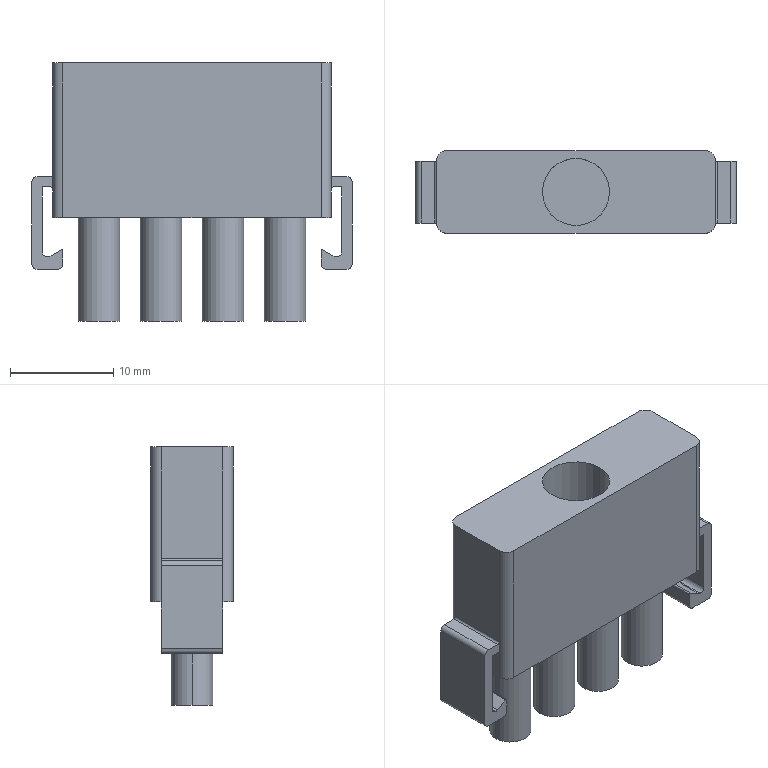Part | SolidWorks | features BaseBody 1 | 1 solid | 87 faces | box 31 x 8 x 25 mm | volume 3494 mm3 | cylinder 48 | plane 39 | commonest cylinder face diameters 2 x12 1 x10 2.5 x8 4 x8 0.2 x4 0.4 x4